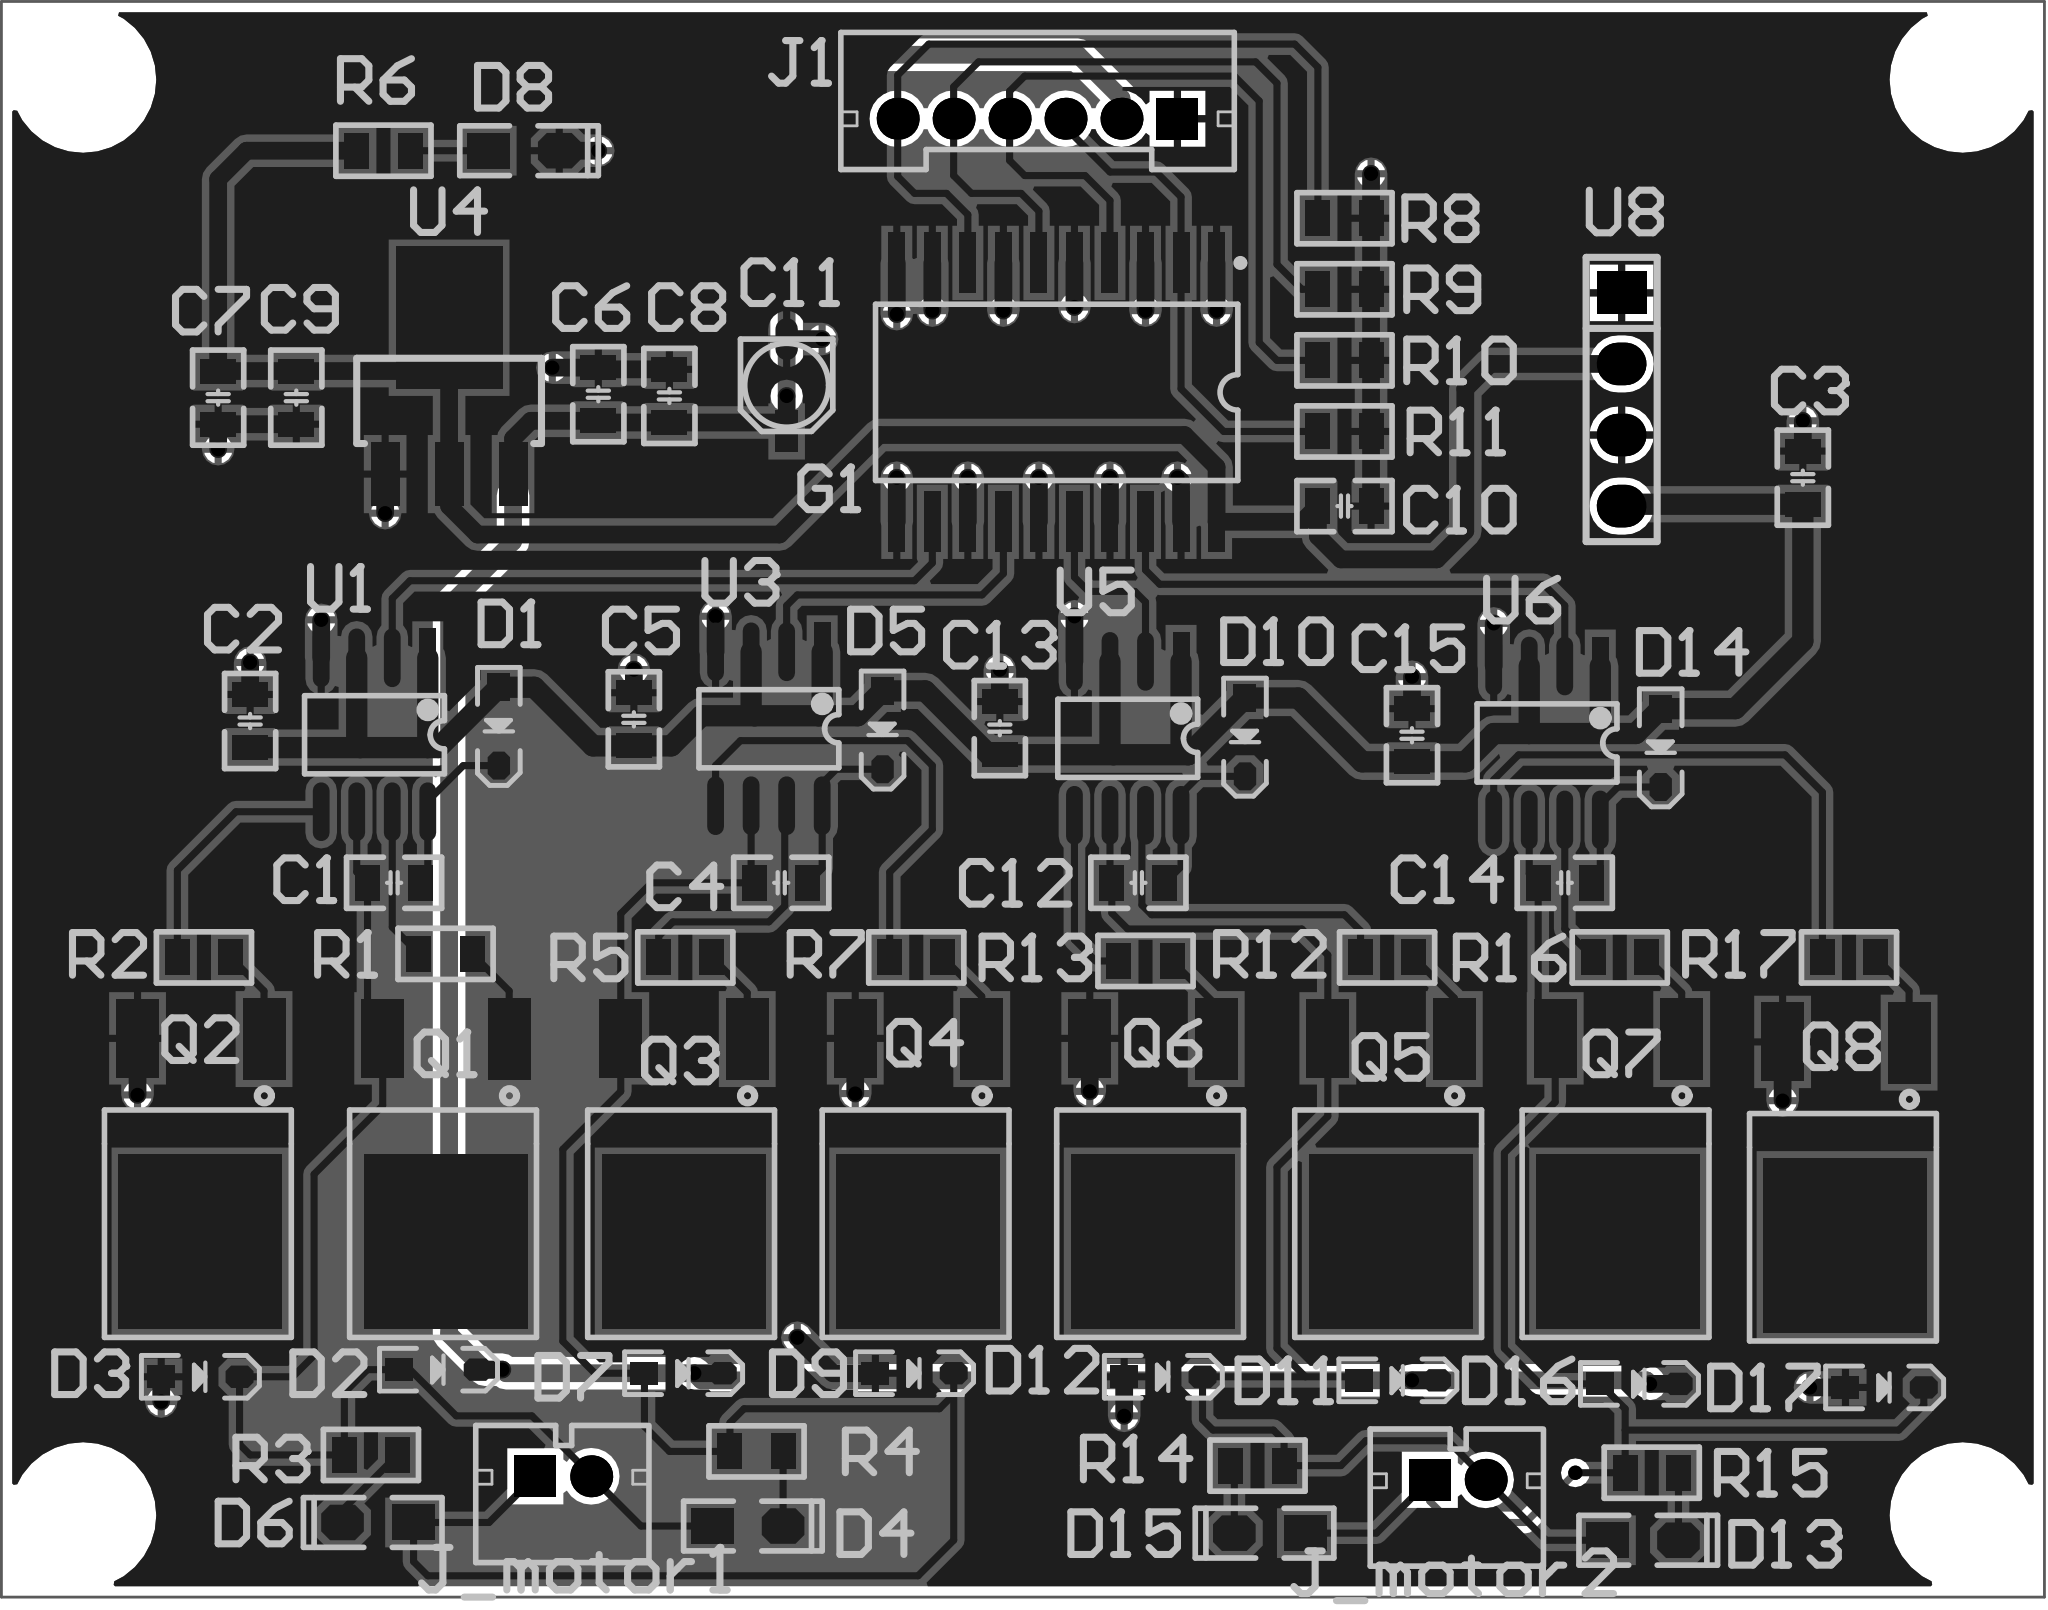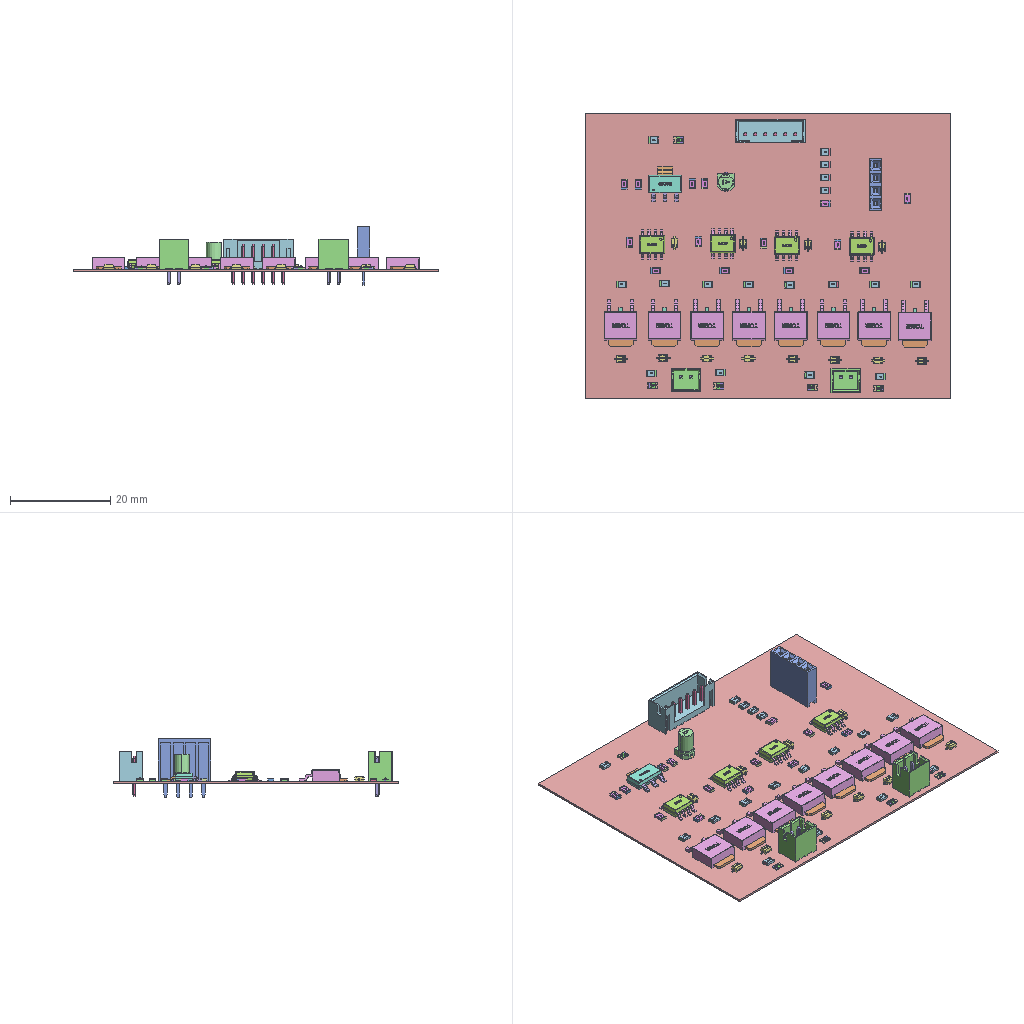Circuit board layout | Altium Designer | box 73 x 57 x 11.7 mm
Layer stack:
# Altium Designer layer stack of  (unit mm; dielectric type: 0 none, 1 core, 2 prepreg, 3 surface material)
index,name,kind,layer,copper_thickness_mm,dielectric_type,dielectric_thickness_mm,dielectric_material,dielectric_constant
0,Top Paste,other,,,,,,
1,Top Overlay,other,,,,,,
2,Top Solder,dielectric,,,3,0.0102,Solder Resist,3.5
3,Top Layer,copper,Top Layer,0.0356,,,,
4,Dielectric 1,dielectric,,,0,0.32,FR-4,4.8
5,Bottom Layer,copper,Bottom Layer,0.0356,,,,
6,Bottom Solder,dielectric,,,3,0.0102,Solder Resist,3.5
7,Bottom Overlay,other,,,,,,
8,Bottom Paste,other,,,,,,
# drill layer pairs: low layer,high layer
drill_pair,Top Layer,Bottom Layer
Part placement:
Designator,Comment,Layer,Footprint,Center-X(mm),Center-Y(mm),Rotation
U8,BL0512,TopLayer,Fe-HDR1X4/2.54-S,83.312,68.199,360
U6,IR2104S,TopLayer,SOP8,80.645,55.924,270
U5,IR2104S,TopLayer,SOP8,65.659,56.09,270
U4,AMS1117,TopLayer,SOT223,41.402,68.326,0
U3,IR2104S,TopLayer,SOP8,52.832,56.432,270
U1,IR2104S,TopLayer,SOP8,38.735,56.217,270
R17,20R,TopLayer,R_0805_L,91.44,48.26,0
R16,20R,TopLayer,R_0805_L,83.246,48.26,0
R15,1K,TopLayer,R_0805_L,84.389,29.845,180
R14,1K,TopLayer,R_0805_L,70.297,30.099,0
R13,20R,TopLayer,R_0805_L,66.294,48.133,0
R12,20R,TopLayer,R_0805_L,74.93,48.26,0
R11,1K,TopLayer,R_0805_L,73.406,67.056,0
R10,1K,TopLayer,R_0805_L,73.406,69.596,0
R9,1K,TopLayer,R_0805_L,73.406,72.136,0
R8,1K,TopLayer,R_0805_L,73.406,74.676,0
R7,20R,TopLayer,R_0805_L,58.1,48.26,0
R6,1K,TopLayer,R_0805_L,39.055,77.089,0
R5,20R,TopLayer,R_0805_L,49.845,48.26,0
R4,1K,TopLayer,R_0805_L,52.39,30.607,180
R3,1K,TopLayer,R_0805_L,38.608,30.48,180
R2,20R,TopLayer,R_0805_L,32.639,48.26,360
R1,20R,TopLayer,R_0805_L,41.275,48.387,0
Q8,MOSFET-N4,TopLayer,TO252,91.327,41.607,180
Q7,MOSFET-N4,TopLayer,TO252,83.199,41.734,180
Q6,MOSFET-N4,TopLayer,TO252,66.562,41.734,180
Q5,MOSFET-N4,TopLayer,TO252,75.071,41.734,180
Q4,MOSFET-N4,TopLayer,TO252,58.18,41.734,180
Q3,MOSFET-N4,TopLayer,TO252,49.798,41.734,180
Q2,MOSFET-N4,TopLayer,TO252,32.526,41.734,180
Q1,MOSFET-N4,TopLayer,TO252,41.289,41.734,180
J_motor2,CON2,TopLayer,PH2.0-2P,77.454,29.591,360
J_motor1,CON2,TopLayer,PH2.0-2P,45.482,29.718,360
J1,CON6,TopLayer,PH2.0-6P,62.436,78.232,180
G1,SN74HC244DW,TopLayer,DW020,63.119,68.453,180
D17,1N5819,TopLayer,SOD-323,92.713,32.893,360
D16,1N5819,TopLayer,SOD-323,83.95,33.02,360
D15,Red,TopLayer,LED_0805G,70.739,27.686,180
D14,1N5819,TopLayer,SOD-323,84.709,55.75,270
D13,Red,TopLayer,LED_0805G,84.074,27.432,360
D12,1N5819,TopLayer,SOD-323,66.932,33.274,360
D11,1N5819,TopLayer,SOD-323,75.314,33.147,360
D10,1N5819,TopLayer,SOD-323,69.85,56.131,270
D9,1N5819,TopLayer,SOD-323,58.039,33.401,360
D8,Red,TopLayer,LED_0805G,44.069,77.089,360
D7,1N5819,TopLayer,SOD-323,49.784,33.401,360
D6,Red,TopLayer,LED_0805G,38.862,28.067,180
D5,1N5819,TopLayer,SOD-323,56.896,56.385,270
D4,Red,TopLayer,LED_0805G,52.07,27.94,360
D3,1N5819,TopLayer,SOD-323,32.512,33.274,360
D2,1N5819,TopLayer,SOD-323,41.024,33.528,360
D1,1N5819,TopLayer,SOD-323,43.18,56.515,270
C15,10UF,TopLayer,C_0805_L,75.819,56.2,270
C14,1.5UF,TopLayer,C_0805_L,81.28,50.927,0
C13,10UF,TopLayer,C_0805_L,61.087,56.454,270
C12,1.5UF,TopLayer,C_0805_L,66.04,50.927,0
C11,470UF,TopLayer,CM_A(3*5.4),53.467,68.707,270
C10,0.1UF,TopLayer,C_0805_L,73.406,64.389,180
C9,10UF,TopLayer,C_0805_L,35.941,68.265,90
C8,10UF,TopLayer,C_0805_L,49.276,68.326,270
C7,0.1UF,TopLayer,C_0805_L,33.147,68.265,90
C6,0.1UF,TopLayer,C_0805_L,46.736,68.387,270
C5,10UF,TopLayer,C_0805_L,48.006,56.769,270
C4,1.5UF,TopLayer,C_0805_L,53.274,50.927,0
C3,10uF,TopLayer,C_0805_L,89.789,65.405,90
C2,10UF,TopLayer,C_0805_L,34.29,56.708,270
C1,1.5UF,TopLayer,C_0805_L,39.436,50.927,0
Pad and via stacks:
# Altium Designer via and pad stacks of  (unit mm). Each distinct definition once, with the count of objects using it.
# via: kind,start_layer,end_layer,hole_mm,diameter_mm,mode(0 simple;1 top-mid-bottom;2 full stack),diameter_per_layer,count,example_net
# pad: kind,layer,hole_mm,hole_type(0 round;1 square;2 slot),plating,top_size,top_shape(1 round;2 rect;3 octagon;9 rounded rect),mid_size,bottom_size,mode,footprint,size_per_layer,count,example
pad,Top Layer,0,0,unplated,6.223x5.842,2,6.223x5.842,6.223x5.842,0,TO252,,8,Q5.2
pad,Top Layer,0,0,unplated,2.794x1.524,2,2.794x1.524,2.794x1.524,0,TO252,,8,Q5.3
pad,Top Layer,0,0,unplated,2.921x1.524,2,2.921x1.524,2.921x1.524,0,TO252,,8,Q5.1
pad,Top Layer,0,0,plated,1x0.8,3,1x0.8,1x0.8,0,SOD-323,,12,D10.2
pad,Top Layer,0,0,plated,1x0.8,2,1x0.8,1x0.8,0,SOD-323,,12,D10.1
pad,Top Layer,0,0,plated,1.27x0.889,2,1.27x0.889,1.27x0.889,0,R 0805_L,,34,R12.1
pad,Top Layer,0,0,plated,0.6x2.1,1,0.6x2.1,0.6x2.1,0,SOP8,,28,U5.5
pad,Top Layer,0,0,plated,0.6x2.1,2,0.6x2.1,0.6x2.1,0,SOP8,,4,U5.1
pad,Top Layer,0,0,plated,1.27x0.889,2,1.27x0.889,1.27x0.889,0,C 0805_L,,28,C12.1
pad,Top Layer,0,0,plated,1.524x1.27,2,1.524x1.27,1.524x1.27,0,LED 0805G,,5,D13.1
pad,Top Layer,0,0,plated,1.524x1.27,3,1.524x1.27,1.524x1.27,0,LED 0805G,,5,D13.2
pad,Top Layer,0,0,plated,1.016x2.286,2,1.016x2.286,1.016x2.286,0,SOT223,,3,U4.3
pad,Top Layer,0,0,plated,3.81x5.08,2,3.81x5.08,3.81x5.08,0,SOT223,,1,U4.2
pad,Top Layer,0,0,plated,1.5x0.8,2,1.5x0.8,1.5x0.8,0,CM A(3*5.4),,1,C11.1
pad,Top Layer,0,0,plated,1.5x0.8,1,1.5x0.8,1.5x0.8,0,CM A(3*5.4),,1,C11.2
pad,Top Layer,0,0,plated,2.15x0.6,2,2.15x0.6,2.15x0.6,0,DW020,,20,G1.1
pad,Multi-Layer,0.8,0,plated,1.5x1.5,2,1.5x1.5,1.5x1.5,0,PH2.0-2P,,2,J_motor1.1
pad,Multi-Layer,0.8,0,plated,1.5x1.5,1,1.5x1.5,1.5x1.5,0,PH2.0-2P,,2,J_motor1.2
pad,Multi-Layer,0.8,0,plated,1.5x1.5,1,1.5x1.5,1.5x1.5,0,PH2.0-6P,,5,J1.5
pad,Multi-Layer,0.8,0,plated,1.5x1.5,2,1.5x1.5,1.5x1.5,0,PH2.0-6P,,1,J1.1
pad,Multi-Layer,0.8128,0,plated,1.524x1.778,1,1.524x1.778,1.524x1.778,0,Fe-HDR1X4/2.54-S,,3,U8.4
pad,Multi-Layer,0.8128,0,plated,1.524x1.778,2,1.524x1.778,1.524x1.778,0,Fe-HDR1X4/2.54-S,,1,U8.1
via,Top Layer,Bottom Layer,0.254,0.508,0,,41,GND
Copper pours:
name,layer,net,type(0 solid;1 hatched;2 none)
D,Top Layer,GND,0
D,Bottom Layer,GND,0
Design rules, without the lines most boards share:
# Altium Designer design rules of  (exported by Altium Designer, unit mm)
# columns: name | kind | enabled | priority | scope1 | scope2 | descriptor | typed fields (field=value)
Clearance | 0 | enabled | 1 | All | All | Clearance Constraint (Gap=10mil) (All),(All) | gap=0.254
PlaneConnect | 6 | enabled | 1 | All | All | Power Plane Connect Rule(Relief Connect )(Expansion=20mil) (Conductor Width=10mil) (Air Gap=10mil) (Entries=4) (All) | relief_conductor_width=0.254 relief_entries=4 relief_expansion=0.508
PolygonConnect | 20 | enabled | 1 | All | All | Polygon Connect Rule(Relief Connect )(Conductor Width=10mil) (Relief Angle=90 Angle) (Entries=4) (Air Gap Width=10mil) (All),(All) | connect_style(0=relief,1=direct,2=none)=0 relief_conductor_width=0.254 relief_entries=4
Width | 2 | enabled | 1 | All | All | Width Constraint (Min=10mil) (Max=1181.102mil) (Preferred=10mil) (All) |
RoutingVias | 11 | enabled | 1 | All | All | Routing Via (MinHoleWidth=28mil) (MaxHoleWidth=28mil) (PreferredHoleWidth=28mil) (MinWidth=50mil) (MaxWidth=50mil) (PreferedWidth=50mil) (All) | via_min_hole=0.7112 via_max_hole=0.7112 via_preferred_diameter=1.27 via_preferred_hole=0.7112
PasteMaskExpansion | 14 | enabled | 1 | All | All | Paste Mask Expansion (Expansion =0mil) (All) | expansion=0
SolderMaskExpansion | 13 | enabled | 1 | All | All | Solder Mask Expansion (Expansion =4mil) (All) | expansion=0.1016
DiffPairsRouting | 51 | enabled | 1 | All | All | Differential Pairs Uncoupled Length using the Gap Constraints (Min=10mil) (Max=10mil) (Prefered=10mil)  and Width Constraints (Min=15mil) (Max=15mil) (Prefered=15mil) (All) |
HoleToHoleClearance | 52 | enabled | 1 | All | All | Hole To Hole Clearance (Gap=10mil) (All),(All) | gap=0.254
MinimumSolderMaskSliver | 53 | enabled | 1 | All | All | Minimum Solder Mask Sliver (Gap=0mil) (All),(All) |
SilkToSolderMaskClearance | 54 | enabled | 1 | IsPad | All | Silk To Solder Mask (Clearance=0mil) (IsPad),(All) |
SilkToSilkClearance | 55 | enabled | 1 | All | All | Silk to Silk (Clearance=0mil) (All),(All) |
Classes set for this board:
# Altium Designer classes of  (member kind: 0 net, 1 component, 2 from-to, 3 pad, 4 layer, 5 differential pair, 6 design channel, 7 polygon, 8 structure, 9 xSignal)
# columns: class name | member kind | superclass | members
Sheet1 | 1 | no | C1; C2; C3; C4; C5; C6; C7; C8; C9; C10; C11; C12; C13; C14; C15; D1; D2; D3; D4; D5; D6; D7; D8; D9; D10; D11; D12; D13; D14; D15; D16; D17; G1; J1; J_motor1; J_motor2; Q1; Q2; Q3; Q4; Q5; Q6; Q7; Q8; R1; R2; R3; R4; R5; R6; R7; R8; R9; R10; R11; R12; R13; R14; R15; R16; R17; U1; U3; U4; U5; U6; U8;